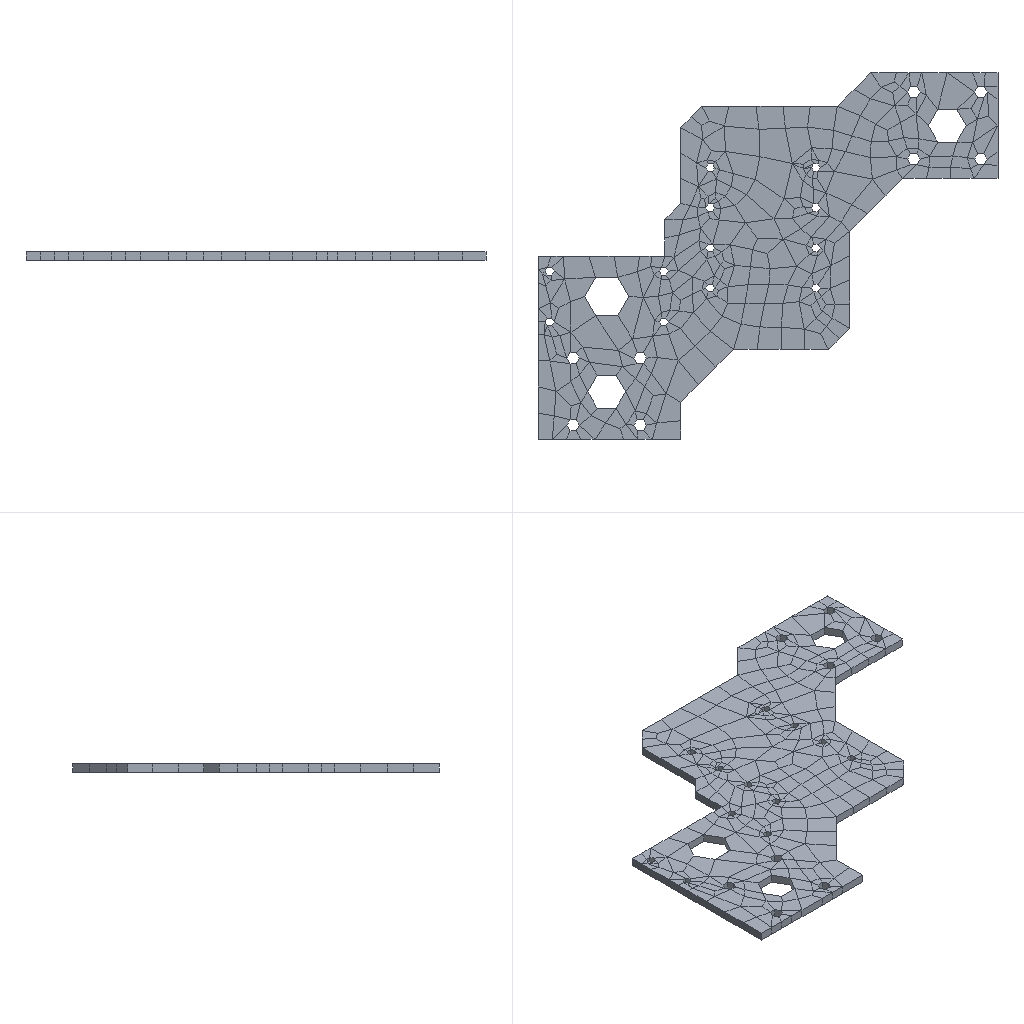Simulation study | ansys workbench
Ansys APDL input file, long lists of numbers shortened:
/batch
/config,noeldb,1     ! force off writing results to database
*get,_wallstrt,active,,time,wall
! ANSYS input file written by Workbench version 2022 R1
! File used for geometry attach: F:\ansys（分析文件汇总)\轴机械结构有限元分析\交付(1)\交付\输出轴.STEP
/title,wbnew--____ (D5)
! ****** Begin Custom Load Command Snippet ******
/COM, ACT Extensions:
/COM,     LSDYNA, 2021.1
/COM,
! ****** End   Custom Load Command Snippet ******
*DIM,_wb_ProjectScratch_dir,string,248
_wb_ProjectScratch_dir(1) = 'C:\Users\Administrator\AppData\Local\Temp\WB_Administrator_11372_2\_ProjectScratch\ScrF44C\'
*DIM,_wb_SolverFiles_dir,string,248
_wb_SolverFiles_dir(1) = 'C:\Users\Administrator\AppData\Local\Temp\WB_Administrator_11372_2\wbnew_files\dp0\SYS-1\MECH\'
*DIM,_wb_userfiles_dir,string,248
_wb_userfiles_dir(1) = 'C:\Users\Administrator\AppData\Local\Temp\WB_Administrator_11372_2\wbnew_files\user_files\'
/com,--- Data in consistent NMM units. See Solving Units in the help system for more information.
/units,MPA
/nopr
/wb,file,start              !  signify a WB generated input file
/prep7
! Turn off shape checking because checks already performed inside WB mesher.
! See help system for more information.
SHPP,OFF,,NOWARN
/nolist
etcon,set             ! allow ANSYS to choose best KEYOP's for 180x elements, resets any applicable keyopt to MAPDL defaults
/com,*********** Nodes for the whole assembly ***********
nblock,3,,7232
(1i9,3e20.9e3)
        1     4.160000000E+01     1.350000000E+01     1.683889349E-15
! (6574 more lines like these left out)
-1
/com,*********** Nodes for all Remote Points ***********
nblock,3
(1i9,3e20.9e3)
     6576    -1.458554756E+01     1.467642368E-07    -9.921145829E-02
-1
/wb,elem,start            !  set before creation of elements
/com,*********** Elements for Body 1 "___-FreeParts|NONE" ***********
et,1,187
eblock,19,solid,,3574
(19i9)
        1        1        1        1        0        0        0        0       10        0        1      728     1089      729     1036     5114     5122     5108     5112
! (7147 more lines like these left out)
-1
/wb,elem,end               !  done creating elements
/com,*********** Send User Defined Coordinate System(s) ***********
csys,0
toffst,273.15,  ! Temperature offset from absolute zero
/com,*********** Set Reference Temperature ***********
tref,22.
/wb,mat,start              !  starting to send materials
/com,*********** Send Materials ***********
Temperature = 'TEMP' ! Temperature
MP,DENS,1,7.85e-09,	! tonne mm^-3
MP,ALPX,1,1.2e-05,	! C^-1
MP,C,1,434000000,	! mm^2 s^-2 C^-1
MP,KXX,1,60.5,	! tonne mm s^-3 C^-1
MP,RSVX,1,0.00017,	! ohm mm
MP,EX,1,200000,	! tonne s^-2 mm^-1
MP,NUXY,1,0.3,
MP,MURX,1,10000,
/wb,mat,end                !  done sending materials
!************************* Model Summary ********************
!___-FreeParts|NONE,	结构钢,	matid,	1
!************************* End Model Summary ********************
! get the diagonal of the bounding box. Needed later for other things
*get,_xmin,node,,mnloc,x
*get,_ymin,node,,mnloc,y
*get,_zmin,node,,mnloc,z
*get,_xmax,node,,mxloc,x
*get,_ymax,node,,mxloc,y
*get,_zmax,node,,mxloc,z
_ASMDIAG=(_xmax-_xmin)*(_xmax-_xmin)+(_ymax-_ymin)*(_ymax-_ymin)+(_zmax-_zmin)*(_zmax-_zmin)
_ASMDIAG=SQRT(_ASMDIAG)
/wb,contact,start          !  starting to send contact
/wb,contact,end            !  done creating contacts
/golist
/wb,load,start             !  starting to send loads
/com,*********** Fixed Supports ***********
CMBLOCK,_FIXEDSU,NODE,      154
(8i10)
       173       174       175       176       177       178       179       180
! (19 more lines like these left out)
cmsel,s,_FIXEDSU
d,all,all
nsel,all
/com,*********** Create Remote Point "内部远程点" ***********
! -------- Remote Point Used by "力矩" --------
*set,tid,3
*set,cid,2
et,cid,174
et,tid,170
keyo,tid,2,1               ! Don't fix the pilot node
keyo,tid,4,111111
keyo,cid,12,5              ! Bonded Contact
keyo,cid,4,1               ! Deformable RBE3 style load
keyo,cid,2,2               ! MPC style contact
eblock,10,,,654
(15i9)
     5224        2        2        2        0      609      161      423      423     1891     1890      423     3704
! (653 more lines like these left out)
-1
*set,_npilot,6576
_npilot32=_npilot
type,tid
mat ,cid
real,cid
tshape,pilo
en,5878,_npilot
tshape
/com,*********** Construct Moment Using Remote Attachment ***********
/gst,on,on
fini
*get,_numnode,node,0,count
*get,_numelem,elem,0,count
*get, _MAXELEMNUM, elem, 0, NUM, MAX
*get, _MAXNODENUM, node, 0, NUM, MAX
*get, _MAXELEMTYPE, etyp, 0, NUM, MAX
*get, _MAXREALCONST, real, 0, NUM, MAX
/go
/wb,load,end               !  done creating loads
/com,--- Number of total nodes = %_numnode%
/com,--- Number of contact elements = 654
/com,--- Number of spring elements = 0
/com,--- Number of bearing elements = 0
/com,--- Number of solid elements = 3574
/com,--- Number of condensed parts = 0
/com,--- Number of total elements = %_numelem%
*get,_wallbsol,active,,time,wall
/com,****************************************************************************
/com,*************************    SOLUTION       ********************************
/com,****************************************************************************
/solu
antype,0                   ! static analysis
_thickRatio=  1     ! Ratio of thick parts in the model
eqsl,pcg,1e-8,,,,,,1
cntr,print,1               ! print out contact info and also make no initial contact an error
dmpoption,emat,no             ! Don't combine emat file for DANSYS
dmpoption,esav,no             ! Don't combine esav file for DANSYS
nldiag,cont,iter           ! print out contact info each equilibrium iteration
rescontrol,,none                 ! Do not keep any restart files
/com,****************************************************
/com,******************* SOLVE FOR LS 1 OF 1 ****************
nsel,s,node,,6576
f,all,mx,8000.
f,all,my,0.
f,all,mz,0.
nsel,all
/nopr
/gopr
nsub,1,1,1
time,1.
outres,erase
outres,all,none
outres,nsol,all,
outres,rsol,all
outres,eangl,all
outres,etmp,all
outres,veng,all
outres,strs,all,
outres,epel,all,
outres,eppl,all,
outres,cont,all,
! *********** WB SOLVE COMMAND ***********
! check interactive state
*get,ANSINTER_,active,,int
*if,ANSINTER_,ne,0,then
/eof
*endif
solve
/com *************** Write FE CONNECTORS *********
CEWRITE,file,ce,,INTE
/com,****************************************************
/com,*************** FINISHED SOLVE FOR LS 1 *************
*get,_wallasol,active,,time,wall
/nopr
*get,_numnode,node,0,count
*get,_numelem,elem,0,count
*get, _MAXELEMNUM, elem, 0, NUM, MAX
*get, _MAXNODENUM, node, 0, NUM, MAX,,,INTERNAL
*get, _MAXELEMTYPE, etyp, 0, NUM, MAX
*get, _MAXREALCONST, real, 0, NUM, MAX
/gopr
*get,_PCGITER,active,,solu,cgiter
/post1
xmlo,ENCODING,ISO-8859-1
xmlo,parm
/xml,parm,xml
fini
/gopr
*get,_walldone,active,,time,wall
_preptime=(_wallbsol-_wallstrt)*3600
_solvtime=(_wallasol-_wallbsol)*3600
_posttime=(_walldone-_wallasol)*3600
_totaltim=(_walldone-_wallstrt)*3600
*get,_dlbratio,active,0,solu,dlbr
*get,_combtime,active,0,solu,comb
*get,_ssmode,active,0,solu,ssmm
*get,_ndofs,active,0,solu,ndof
*get,_sol_end_time,active,0,set,time
*if,_sol_end_time,eq,1.,then
/fclean				!clean distributed files
*endif
/com,--- Total number of nodes = %_numnode%
/com,--- Total number of elements = %_numelem%
/com,--- Element load balance ratio = %_dlbratio%
/com,--- Time to combine distributed files = %_combtime%
/com,--- Sparse memory mode = %_ssmode%
/com,--- Number of DOF = %_ndofs%
/wb,file,end               ! done with WB generated input